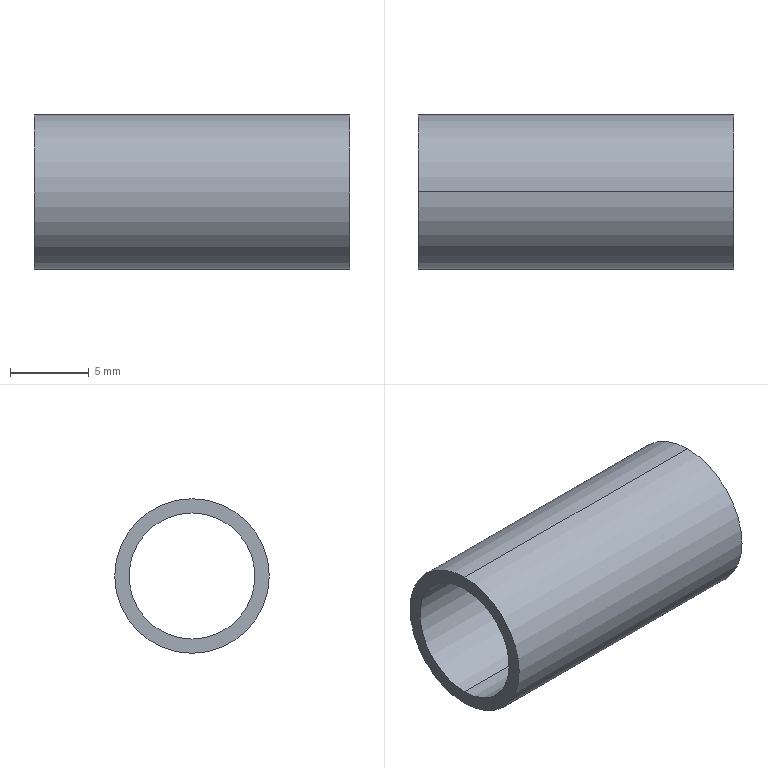Part | SolidWorks | features RefAxis 3, 3DProfileFeature 1, Revolution 1 | 1 solid | 6 faces | box 20 x 9.8 x 9.8 mm | volume 503.283 mm3 | cylinder 4 | plane 2 | commonest cylinder face diameters 8 x2 9.8 x2
STEP:
#1=CARTESIAN_POINT('',(10.,0.,-4.));
#2=VERTEX_POINT('',#1);
#3=CARTESIAN_POINT('',(10.,0.,4.));
#4=VERTEX_POINT('',#3);
#5=CARTESIAN_POINT('',(10.,0.,0.));
#6=DIRECTION('',(-1.,0.,0.));
#7=DIRECTION('',(0.,0.,1.));
#8=AXIS2_PLACEMENT_3D('',#5,#6,#7);
#9=CIRCLE('',#8,4.);
#10=EDGE_CURVE('',#2,#4,#9,.T.);
#11=ORIENTED_EDGE('',*,*,#10,.F.);
#12=CARTESIAN_POINT('',(-10.,0.,-4.));
#13=VERTEX_POINT('',#12);
#14=CARTESIAN_POINT('',(10.,0.,-4.));
#15=DIRECTION('',(-1.,0.,0.));
#16=VECTOR('',#15,1000.);
#17=LINE('',#14,#16);
#18=EDGE_CURVE('',#2,#13,#17,.T.);
#19=ORIENTED_EDGE('',*,*,#18,.T.);
#20=CARTESIAN_POINT('',(-10.,0.,4.));
#21=VERTEX_POINT('',#20);
#22=CARTESIAN_POINT('',(-10.,0.,0.));
#23=DIRECTION('',(-1.,0.,0.));
#24=DIRECTION('',(0.,0.,1.));
#25=AXIS2_PLACEMENT_3D('',#22,#23,#24);
#26=CIRCLE('',#25,4.);
#27=EDGE_CURVE('',#13,#21,#26,.T.);
#28=ORIENTED_EDGE('',*,*,#27,.T.);
#29=CARTESIAN_POINT('',(10.,0.,4.));
#30=DIRECTION('',(-1.,0.,0.));
#31=VECTOR('',#30,1000.);
#32=LINE('',#29,#31);
#33=EDGE_CURVE('',#4,#21,#32,.T.);
#34=ORIENTED_EDGE('',*,*,#33,.F.);
#35=EDGE_LOOP('',(#11,#19,#28,#34));
#36=FACE_OUTER_BOUND('',#35,.T.);
#37=CARTESIAN_POINT('',(10.,0.,0.));
#38=DIRECTION('',(-1.,0.,0.));
#39=DIRECTION('',(0.,0.,1.));
#40=AXIS2_PLACEMENT_3D('',#37,#38,#39);
#41=CYLINDRICAL_SURFACE('',#40,4.);
#42=ADVANCED_FACE('',(#36),#41,.F.);
#43=CARTESIAN_POINT('',(10.,0.,4.9));
#44=VERTEX_POINT('',#43);
#45=CARTESIAN_POINT('',(10.,0.,-4.9));
#46=VERTEX_POINT('',#45);
#47=CARTESIAN_POINT('',(10.,0.,0.));
#48=DIRECTION('',(-1.,0.,0.));
#49=DIRECTION('',(0.,0.,1.));
#50=AXIS2_PLACEMENT_3D('',#47,#48,#49);
#51=CIRCLE('',#50,4.9);
#52=EDGE_CURVE('',#44,#46,#51,.T.);
#53=ORIENTED_EDGE('',*,*,#52,.T.);
#54=CARTESIAN_POINT('',(-10.,0.,-4.9));
#55=VERTEX_POINT('',#54);
#56=CARTESIAN_POINT('',(10.,0.,-4.9));
#57=DIRECTION('',(-1.,0.,0.));
#58=VECTOR('',#57,1000.);
#59=LINE('',#56,#58);
#60=EDGE_CURVE('',#46,#55,#59,.T.);
#61=ORIENTED_EDGE('',*,*,#60,.T.);
#62=CARTESIAN_POINT('',(-10.,0.,4.9));
#63=VERTEX_POINT('',#62);
#64=CARTESIAN_POINT('',(-10.,0.,0.));
#65=DIRECTION('',(-1.,0.,0.));
#66=DIRECTION('',(0.,0.,1.));
#67=AXIS2_PLACEMENT_3D('',#64,#65,#66);
#68=CIRCLE('',#67,4.9);
#69=EDGE_CURVE('',#63,#55,#68,.T.);
#70=ORIENTED_EDGE('',*,*,#69,.F.);
#71=CARTESIAN_POINT('',(10.,0.,4.9));
#72=DIRECTION('',(-1.,0.,0.));
#73=VECTOR('',#72,1000.);
#74=LINE('',#71,#73);
#75=EDGE_CURVE('',#44,#63,#74,.T.);
#76=ORIENTED_EDGE('',*,*,#75,.F.);
#77=EDGE_LOOP('',(#53,#61,#70,#76));
#78=FACE_OUTER_BOUND('',#77,.T.);
#79=CARTESIAN_POINT('',(10.,0.,0.));
#80=DIRECTION('',(-1.,0.,0.));
#81=DIRECTION('',(0.,0.,1.));
#82=AXIS2_PLACEMENT_3D('',#79,#80,#81);
#83=CYLINDRICAL_SURFACE('',#82,4.9);
#84=ADVANCED_FACE('',(#78),#83,.T.);
#85=ORIENTED_EDGE('',*,*,#60,.F.);
#86=CARTESIAN_POINT('',(10.,0.,0.));
#87=DIRECTION('',(-1.,0.,0.));
#88=DIRECTION('',(0.,0.,1.));
#89=AXIS2_PLACEMENT_3D('',#86,#87,#88);
#90=CIRCLE('',#89,4.9);
#91=EDGE_CURVE('',#46,#44,#90,.T.);
#92=ORIENTED_EDGE('',*,*,#91,.T.);
#93=ORIENTED_EDGE('',*,*,#75,.T.);
#94=CARTESIAN_POINT('',(-10.,0.,0.));
#95=DIRECTION('',(-1.,0.,0.));
#96=DIRECTION('',(0.,0.,1.));
#97=AXIS2_PLACEMENT_3D('',#94,#95,#96);
#98=CIRCLE('',#97,4.9);
#99=EDGE_CURVE('',#55,#63,#98,.T.);
#100=ORIENTED_EDGE('',*,*,#99,.F.);
#101=EDGE_LOOP('',(#85,#92,#93,#100));
#102=FACE_OUTER_BOUND('',#101,.T.);
#103=CARTESIAN_POINT('',(10.,0.,0.));
#104=DIRECTION('',(-1.,0.,0.));
#105=DIRECTION('',(0.,0.,1.));
#106=AXIS2_PLACEMENT_3D('',#103,#104,#105);
#107=CYLINDRICAL_SURFACE('',#106,4.9);
#108=ADVANCED_FACE('',(#102),#107,.T.);
#109=CARTESIAN_POINT('',(-10.,0.,0.));
#110=DIRECTION('',(-1.,0.,0.));
#111=DIRECTION('',(0.,0.,1.));
#112=AXIS2_PLACEMENT_3D('',#109,#110,#111);
#113=CIRCLE('',#112,4.);
#114=EDGE_CURVE('',#21,#13,#113,.T.);
#115=ORIENTED_EDGE('',*,*,#114,.F.);
#116=ORIENTED_EDGE('',*,*,#27,.F.);
#117=EDGE_LOOP('',(#115,#116));
#118=FACE_BOUND('',#117,.T.);
#119=ORIENTED_EDGE('',*,*,#69,.T.);
#120=ORIENTED_EDGE('',*,*,#99,.T.);
#121=EDGE_LOOP('',(#119,#120));
#122=FACE_OUTER_BOUND('',#121,.T.);
#123=CARTESIAN_POINT('',(-10.,4.9,0.));
#124=DIRECTION('',(1.,0.,0.));
#125=DIRECTION('',(0.,0.,-1.));
#126=AXIS2_PLACEMENT_3D('',#123,#124,#125);
#127=PLANE('',#126);
#128=ADVANCED_FACE('',(#118,#122),#127,.F.);
#129=ORIENTED_EDGE('',*,*,#18,.F.);
#130=CARTESIAN_POINT('',(10.,0.,0.));
#131=DIRECTION('',(-1.,0.,0.));
#132=DIRECTION('',(0.,0.,1.));
#133=AXIS2_PLACEMENT_3D('',#130,#131,#132);
#134=CIRCLE('',#133,4.);
#135=EDGE_CURVE('',#4,#2,#134,.T.);
#136=ORIENTED_EDGE('',*,*,#135,.F.);
#137=ORIENTED_EDGE('',*,*,#33,.T.);
#138=ORIENTED_EDGE('',*,*,#114,.T.);
#139=EDGE_LOOP('',(#129,#136,#137,#138));
#140=FACE_OUTER_BOUND('',#139,.T.);
#141=CARTESIAN_POINT('',(10.,0.,0.));
#142=DIRECTION('',(-1.,0.,0.));
#143=DIRECTION('',(0.,0.,1.));
#144=AXIS2_PLACEMENT_3D('',#141,#142,#143);
#145=CYLINDRICAL_SURFACE('',#144,4.);
#146=ADVANCED_FACE('',(#140),#145,.F.);
#147=ORIENTED_EDGE('',*,*,#52,.F.);
#148=ORIENTED_EDGE('',*,*,#91,.F.);
#149=EDGE_LOOP('',(#147,#148));
#150=FACE_OUTER_BOUND('',#149,.T.);
#151=ORIENTED_EDGE('',*,*,#135,.T.);
#152=ORIENTED_EDGE('',*,*,#10,.T.);
#153=EDGE_LOOP('',(#151,#152));
#154=FACE_BOUND('',#153,.T.);
#155=CARTESIAN_POINT('',(10.,4.,0.));
#156=DIRECTION('',(-1.,0.,0.));
#157=DIRECTION('',(0.,0.,1.));
#158=AXIS2_PLACEMENT_3D('',#155,#156,#157);
#159=PLANE('',#158);
#160=ADVANCED_FACE('',(#150,#154),#159,.F.);
#161=CLOSED_SHELL('',(#42,#84,#108,#128,#146,#160));
#162=MANIFOLD_SOLID_BREP('',#161);
#163=CARTESIAN_POINT('',(0.,0.,0.));
#164=DIRECTION('',(0.,0.,1.));
#165=DIRECTION('',(1.,0.,0.));
#166=AXIS2_PLACEMENT_3D('',#163,#164,#165);
#167=(LENGTH_UNIT()NAMED_UNIT(*)SI_UNIT(.MILLI.,.METRE.));
#168=UNCERTAINTY_MEASURE_WITH_UNIT(LENGTH_MEASURE(0.00001),#167,'','');
#169=(NAMED_UNIT(*)PLANE_ANGLE_UNIT()SI_UNIT($,.RADIAN.));
#170=(NAMED_UNIT(*)SI_UNIT($,.STERADIAN.)SOLID_ANGLE_UNIT());
#171=(GEOMETRIC_REPRESENTATION_CONTEXT(3)GLOBAL_UNCERTAINTY_ASSIGNED_CONTEXT((#168))GLOBAL_UNIT_ASSIGNED_CONTEXT((#167,#169,#170))REPRESENTATION_CONTEXT('',''));
#172=ADVANCED_BREP_SHAPE_REPRESENTATION('',(#162,#166),#171);